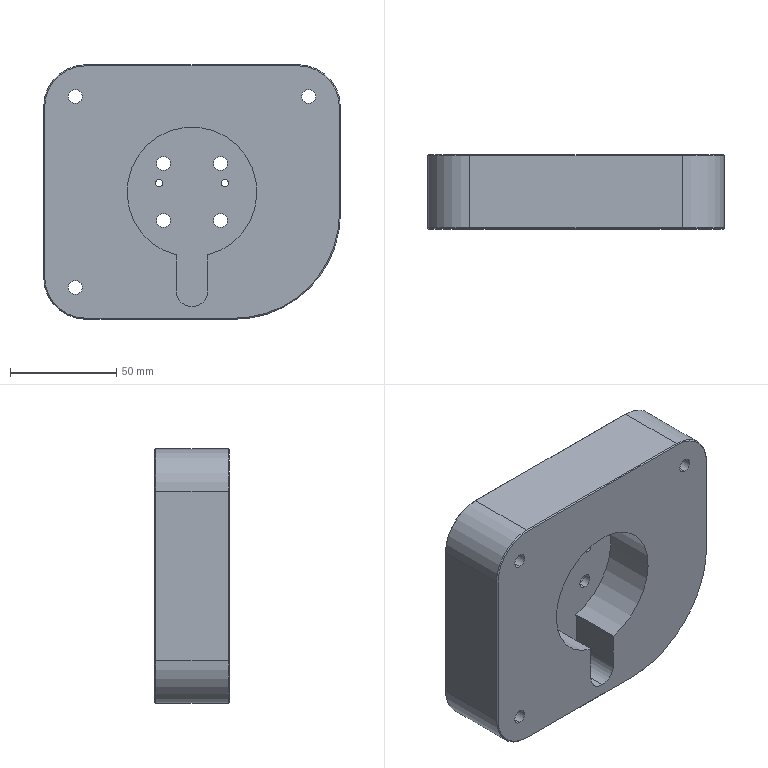Part | STEP file | ND25021-01-JDKM-24-TL | 1 solid | 73 faces | box 140 x 35 x 120 mm | volume 469712 mm3 | cylinder 41 | plane 24 | cone 8 | commonest cylinder face diameters 6.6 x14 11 x14 3.3 x4 15 x4 40 x3 61.2 x1